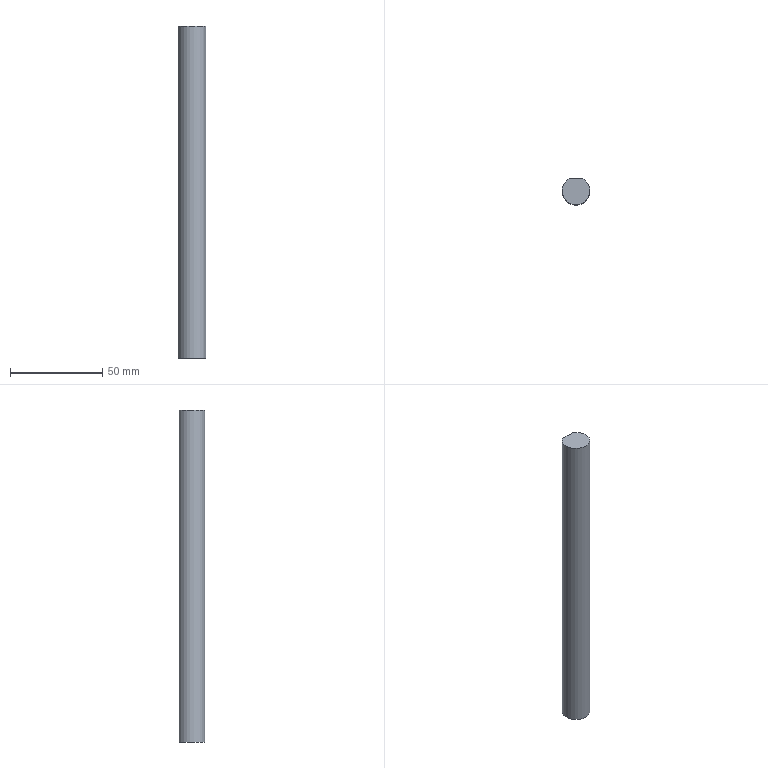Part | NX | 1 solid | 10 faces | box 15 x 14 x 180 mm | volume 30639 mm3 | plane 6 | cylinder 4 | commonest cylinder face diameters 3.3 x3 15 x1
STEP:
#1=CARTESIAN_POINT('',(0.,6.5,168.35));
#2=VERTEX_POINT('',#1);
#3=CARTESIAN_POINT('',(0.,6.5,170.));
#4=DIRECTION('',(0.,1.,0.));
#5=DIRECTION('',(0.,0.,-1.));
#6=AXIS2_PLACEMENT_3D('',#3,#4,#5);
#7=CIRCLE('',#6,1.65);
#8=EDGE_CURVE('',#2,#2,#7,.T.);
#9=ORIENTED_EDGE('',*,*,#8,.F.);
#10=EDGE_LOOP('',(#9));
#11=FACE_BOUND('',#10,.T.);
#12=CARTESIAN_POINT('',(0.,6.5,108.35));
#13=VERTEX_POINT('',#12);
#14=CARTESIAN_POINT('',(0.,6.5,110.));
#15=DIRECTION('',(0.,1.,0.));
#16=DIRECTION('',(0.,0.,-1.));
#17=AXIS2_PLACEMENT_3D('',#14,#15,#16);
#18=CIRCLE('',#17,1.65);
#19=EDGE_CURVE('',#13,#13,#18,.T.);
#20=ORIENTED_EDGE('',*,*,#19,.F.);
#21=EDGE_LOOP('',(#20));
#22=FACE_BOUND('',#21,.T.);
#23=CARTESIAN_POINT('',(0.,6.5,48.35));
#24=VERTEX_POINT('',#23);
#25=CARTESIAN_POINT('',(0.,6.5,50.));
#26=DIRECTION('',(0.,1.,0.));
#27=DIRECTION('',(0.,0.,-1.));
#28=AXIS2_PLACEMENT_3D('',#25,#26,#27);
#29=CIRCLE('',#28,1.65);
#30=EDGE_CURVE('',#24,#24,#29,.T.);
#31=ORIENTED_EDGE('',*,*,#30,.F.);
#32=EDGE_LOOP('',(#31));
#33=FACE_BOUND('',#32,.T.);
#34=CARTESIAN_POINT('',(3.742,6.5,0.));
#35=VERTEX_POINT('',#34);
#36=CARTESIAN_POINT('',(-3.742,6.5,0.));
#37=VERTEX_POINT('',#36);
#38=CARTESIAN_POINT('',(3.742,6.5,0.));
#39=DIRECTION('',(-1.,0.,0.));
#40=VECTOR('',#39,1000.);
#41=LINE('',#38,#40);
#42=EDGE_CURVE('',#35,#37,#41,.T.);
#43=ORIENTED_EDGE('',*,*,#42,.T.);
#44=CARTESIAN_POINT('',(-3.742,6.5,180.));
#45=VERTEX_POINT('',#44);
#46=CARTESIAN_POINT('',(-3.742,6.5,180.));
#47=DIRECTION('',(0.,0.,-1.));
#48=VECTOR('',#47,1000.);
#49=LINE('',#46,#48);
#50=EDGE_CURVE('',#45,#37,#49,.T.);
#51=ORIENTED_EDGE('',*,*,#50,.F.);
#52=CARTESIAN_POINT('',(3.742,6.5,180.));
#53=VERTEX_POINT('',#52);
#54=CARTESIAN_POINT('',(3.742,6.5,180.));
#55=DIRECTION('',(-1.,0.,0.));
#56=VECTOR('',#55,1000.);
#57=LINE('',#54,#56);
#58=EDGE_CURVE('',#53,#45,#57,.T.);
#59=ORIENTED_EDGE('',*,*,#58,.F.);
#60=CARTESIAN_POINT('',(3.742,6.5,180.));
#61=DIRECTION('',(0.,0.,-1.));
#62=VECTOR('',#61,1000.);
#63=LINE('',#60,#62);
#64=EDGE_CURVE('',#35,#53,#63,.F.);
#65=ORIENTED_EDGE('',*,*,#64,.F.);
#66=EDGE_LOOP('',(#43,#51,#59,#65));
#67=FACE_BOUND('',#66,.T.);
#68=CARTESIAN_POINT('',(3.742,6.5,180.));
#69=DIRECTION('',(0.,-1.,0.));
#70=DIRECTION('',(0.,0.,-1.));
#71=AXIS2_PLACEMENT_3D('',#68,#69,#70);
#72=PLANE('',#71);
#73=ADVANCED_FACE('',(#11,#22,#33,#67),#72,.F.);
#74=CARTESIAN_POINT('',(0.,0.,0.));
#75=DIRECTION('',(0.,0.,1.));
#76=DIRECTION('',(1.,0.,0.));
#77=AXIS2_PLACEMENT_3D('',#74,#75,#76);
#78=CIRCLE('',#77,7.5);
#79=EDGE_CURVE('',#37,#35,#78,.T.);
#80=ORIENTED_EDGE('',*,*,#79,.T.);
#81=ORIENTED_EDGE('',*,*,#64,.T.);
#82=CARTESIAN_POINT('',(0.,0.,180.));
#83=DIRECTION('',(0.,0.,1.));
#84=DIRECTION('',(1.,0.,0.));
#85=AXIS2_PLACEMENT_3D('',#82,#83,#84);
#86=CIRCLE('',#85,7.5);
#87=EDGE_CURVE('',#45,#53,#86,.T.);
#88=ORIENTED_EDGE('',*,*,#87,.F.);
#89=ORIENTED_EDGE('',*,*,#50,.T.);
#90=EDGE_LOOP('',(#80,#81,#88,#89));
#91=FACE_BOUND('',#90,.T.);
#92=CARTESIAN_POINT('',(0.,0.,180.));
#93=DIRECTION('',(0.,0.,-1.));
#94=DIRECTION('',(-1.,0.,0.));
#95=AXIS2_PLACEMENT_3D('',#92,#93,#94);
#96=CYLINDRICAL_SURFACE('',#95,7.5);
#97=ADVANCED_FACE('',(#91),#96,.T.);
#98=ORIENTED_EDGE('',*,*,#58,.T.);
#99=ORIENTED_EDGE('',*,*,#87,.T.);
#100=EDGE_LOOP('',(#98,#99));
#101=FACE_BOUND('',#100,.T.);
#102=CARTESIAN_POINT('',(0.,0.,180.));
#103=DIRECTION('',(0.,0.,1.));
#104=DIRECTION('',(1.,0.,0.));
#105=AXIS2_PLACEMENT_3D('',#102,#103,#104);
#106=PLANE('',#105);
#107=ADVANCED_FACE('',(#101),#106,.T.);
#108=ORIENTED_EDGE('',*,*,#42,.F.);
#109=ORIENTED_EDGE('',*,*,#79,.F.);
#110=EDGE_LOOP('',(#108,#109));
#111=FACE_BOUND('',#110,.T.);
#112=CARTESIAN_POINT('',(0.,0.,0.));
#113=DIRECTION('',(0.,0.,1.));
#114=DIRECTION('',(1.,0.,0.));
#115=AXIS2_PLACEMENT_3D('',#112,#113,#114);
#116=PLANE('',#115);
#117=ADVANCED_FACE('',(#111),#116,.F.);
#118=CARTESIAN_POINT('',(0.,-3.6,48.35));
#119=VERTEX_POINT('',#118);
#120=CARTESIAN_POINT('',(0.,-3.6,50.));
#121=DIRECTION('',(0.,1.,0.));
#122=DIRECTION('',(0.,0.,-1.));
#123=AXIS2_PLACEMENT_3D('',#120,#121,#122);
#124=CIRCLE('',#123,1.65);
#125=EDGE_CURVE('',#119,#119,#124,.F.);
#126=ORIENTED_EDGE('',*,*,#125,.T.);
#127=EDGE_LOOP('',(#126));
#128=FACE_BOUND('',#127,.T.);
#129=ORIENTED_EDGE('',*,*,#30,.T.);
#130=EDGE_LOOP('',(#129));
#131=FACE_BOUND('',#130,.T.);
#132=CARTESIAN_POINT('',(0.,-3.6,50.));
#133=DIRECTION('',(0.,1.,0.));
#134=DIRECTION('',(0.,0.,1.));
#135=AXIS2_PLACEMENT_3D('',#132,#133,#134);
#136=CYLINDRICAL_SURFACE('',#135,1.65);
#137=ADVANCED_FACE('',(#128,#131),#136,.F.);
#138=ORIENTED_EDGE('',*,*,#125,.F.);
#139=EDGE_LOOP('',(#138));
#140=FACE_BOUND('',#139,.T.);
#141=CARTESIAN_POINT('',(0.,-3.6,50.));
#142=DIRECTION('',(0.,1.,0.));
#143=DIRECTION('',(0.,0.,1.));
#144=AXIS2_PLACEMENT_3D('',#141,#142,#143);
#145=PLANE('',#144);
#146=ADVANCED_FACE('',(#140),#145,.T.);
#147=CARTESIAN_POINT('',(0.,-3.6,108.35));
#148=VERTEX_POINT('',#147);
#149=CARTESIAN_POINT('',(0.,-3.6,110.));
#150=DIRECTION('',(0.,1.,0.));
#151=DIRECTION('',(0.,0.,-1.));
#152=AXIS2_PLACEMENT_3D('',#149,#150,#151);
#153=CIRCLE('',#152,1.65);
#154=EDGE_CURVE('',#148,#148,#153,.F.);
#155=ORIENTED_EDGE('',*,*,#154,.T.);
#156=EDGE_LOOP('',(#155));
#157=FACE_BOUND('',#156,.T.);
#158=ORIENTED_EDGE('',*,*,#19,.T.);
#159=EDGE_LOOP('',(#158));
#160=FACE_BOUND('',#159,.T.);
#161=CARTESIAN_POINT('',(0.,-3.6,110.));
#162=DIRECTION('',(0.,1.,0.));
#163=DIRECTION('',(0.,0.,1.));
#164=AXIS2_PLACEMENT_3D('',#161,#162,#163);
#165=CYLINDRICAL_SURFACE('',#164,1.65);
#166=ADVANCED_FACE('',(#157,#160),#165,.F.);
#167=ORIENTED_EDGE('',*,*,#154,.F.);
#168=EDGE_LOOP('',(#167));
#169=FACE_BOUND('',#168,.T.);
#170=CARTESIAN_POINT('',(0.,-3.6,110.));
#171=DIRECTION('',(0.,1.,0.));
#172=DIRECTION('',(0.,0.,1.));
#173=AXIS2_PLACEMENT_3D('',#170,#171,#172);
#174=PLANE('',#173);
#175=ADVANCED_FACE('',(#169),#174,.T.);
#176=CARTESIAN_POINT('',(0.,-3.6,168.35));
#177=VERTEX_POINT('',#176);
#178=CARTESIAN_POINT('',(0.,-3.6,170.));
#179=DIRECTION('',(0.,1.,0.));
#180=DIRECTION('',(0.,0.,-1.));
#181=AXIS2_PLACEMENT_3D('',#178,#179,#180);
#182=CIRCLE('',#181,1.65);
#183=EDGE_CURVE('',#177,#177,#182,.F.);
#184=ORIENTED_EDGE('',*,*,#183,.T.);
#185=EDGE_LOOP('',(#184));
#186=FACE_BOUND('',#185,.T.);
#187=ORIENTED_EDGE('',*,*,#8,.T.);
#188=EDGE_LOOP('',(#187));
#189=FACE_BOUND('',#188,.T.);
#190=CARTESIAN_POINT('',(0.,-3.6,170.));
#191=DIRECTION('',(0.,1.,0.));
#192=DIRECTION('',(0.,0.,1.));
#193=AXIS2_PLACEMENT_3D('',#190,#191,#192);
#194=CYLINDRICAL_SURFACE('',#193,1.65);
#195=ADVANCED_FACE('',(#186,#189),#194,.F.);
#196=ORIENTED_EDGE('',*,*,#183,.F.);
#197=EDGE_LOOP('',(#196));
#198=FACE_BOUND('',#197,.T.);
#199=CARTESIAN_POINT('',(0.,-3.6,170.));
#200=DIRECTION('',(0.,1.,0.));
#201=DIRECTION('',(0.,0.,1.));
#202=AXIS2_PLACEMENT_3D('',#199,#200,#201);
#203=PLANE('',#202);
#204=ADVANCED_FACE('',(#198),#203,.T.);
#205=CLOSED_SHELL('',(#73,#97,#107,#117,#137,#146,#166,#175,#195,#204));
#206=MANIFOLD_SOLID_BREP('',#205);
#207=(LENGTH_UNIT()NAMED_UNIT(*)SI_UNIT(.MILLI.,.METRE.));
#208=UNCERTAINTY_MEASURE_WITH_UNIT(LENGTH_MEASURE(0.00001),#207,'','');
#209=(NAMED_UNIT(*)PLANE_ANGLE_UNIT()SI_UNIT($,.RADIAN.));
#210=(NAMED_UNIT(*)SI_UNIT($,.STERADIAN.)SOLID_ANGLE_UNIT());
#211=(GEOMETRIC_REPRESENTATION_CONTEXT(3)GLOBAL_UNCERTAINTY_ASSIGNED_CONTEXT((#208))GLOBAL_UNIT_ASSIGNED_CONTEXT((#207,#209,#210))REPRESENTATION_CONTEXT('',''));
#212=ADVANCED_BREP_SHAPE_REPRESENTATION('',(#206),#211);